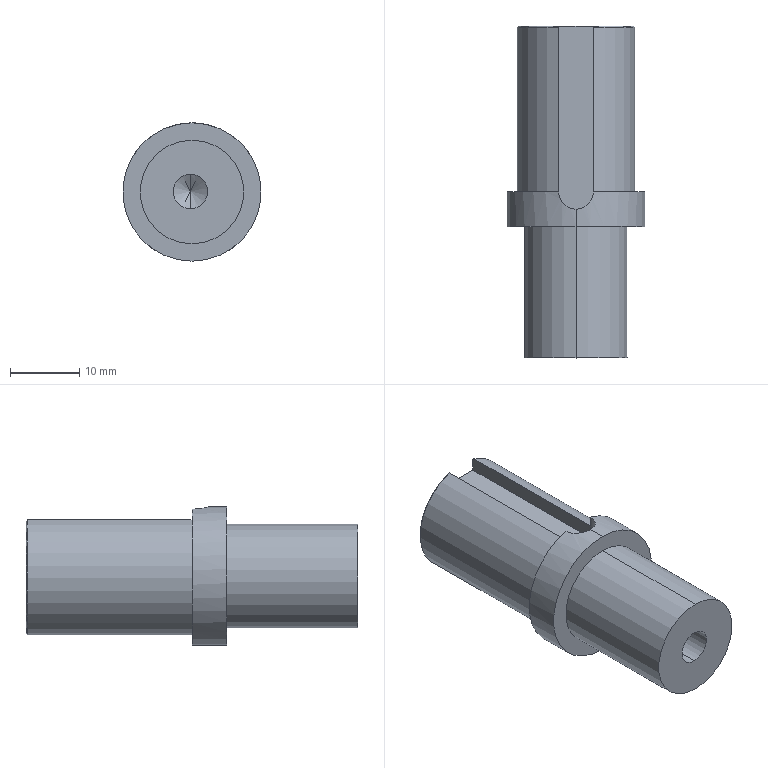Part | STEP file | Cuon T phu H01_9 | 1 solid | 24 faces | box 20 x 48 x 20 mm | volume 9443 mm3 | cylinder 11 | plane 7 | cone 6 | commonest cylinder face diameters 5 x5 15 x2 17 x2 20 x2